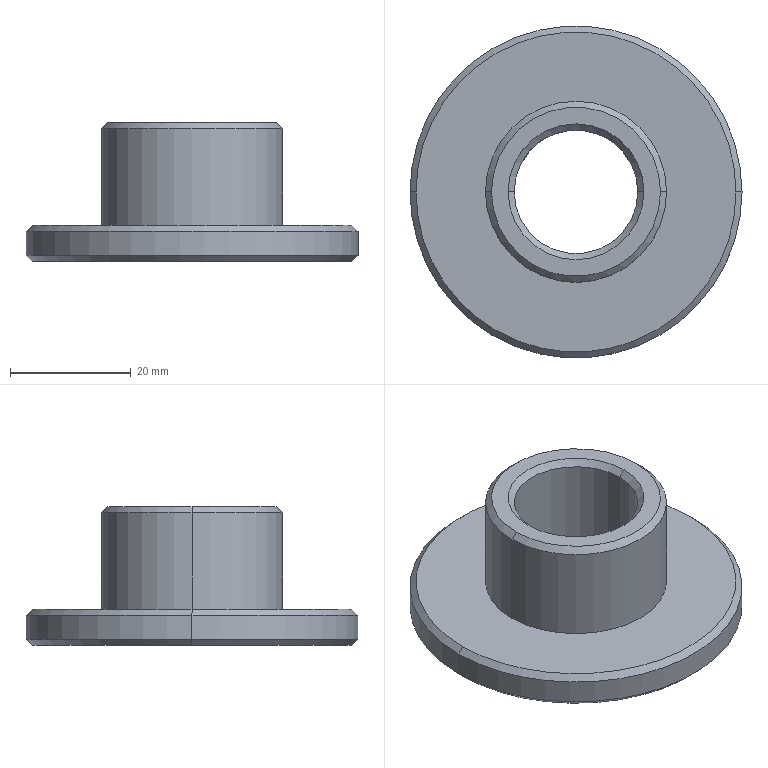Part | STEP file | YCD14007A-08.02.19 Lifting Cylinder Joint Modified | 1 solid | 19 faces | box 55 x 55 x 23 mm | volume 18397 mm3 | cone 10 | cylinder 6 | plane 3 | commonest cylinder face diameters 20.5 x2 30 x2 55 x2
STEP:
#1=CARTESIAN_POINT('',(0.,0.,0.));
#2=DIRECTION('',(0.,0.,1.));
#3=DIRECTION('',(1.,0.,0.));
#4=AXIS2_PLACEMENT_3D('',#1,#2,#3);
#5=CARTESIAN_POINT('',(10.25,0.,10.5));
#6=VERTEX_POINT('',#5);
#7=CARTESIAN_POINT('',(11.25,0.,11.5));
#8=VERTEX_POINT('',#7);
#9=CARTESIAN_POINT('',(10.25,0.,10.5));
#10=DIRECTION('',(0.7071,0.,0.7071));
#11=VECTOR('',#10,1.);
#12=LINE('',#9,#11);
#13=CARTESIAN_POINT('',(0.,0.,10.5));
#14=DIRECTION('',(0.,0.,1.));
#15=DIRECTION('',(1.,0.,0.));
#16=AXIS2_PLACEMENT_3D('',#13,#14,#15);
#17=CONICAL_SURFACE('',#16,10.25,0.7854);
#18=CARTESIAN_POINT('',(6.283,0.));
#19=DIRECTION('',(0.,1.));
#20=VECTOR('',#19,1.);
#21=LINE('',#18,#20);
#22=(GEOMETRIC_REPRESENTATION_CONTEXT(2)PARAMETRIC_REPRESENTATION_CONTEXT()REPRESENTATION_CONTEXT('',''));
#23=DEFINITIONAL_REPRESENTATION('',(#21),#22);
#24=PCURVE('',#17,#23);
#25=CARTESIAN_POINT('',(0.,0.,10.5));
#26=DIRECTION('',(0.,0.,1.));
#27=DIRECTION('',(1.,0.,0.));
#28=AXIS2_PLACEMENT_3D('',#25,#26,#27);
#29=CONICAL_SURFACE('',#28,10.25,0.7854);
#30=CARTESIAN_POINT('',(0.,0.));
#31=DIRECTION('',(0.,1.));
#32=VECTOR('',#31,1.);
#33=LINE('',#30,#32);
#34=(GEOMETRIC_REPRESENTATION_CONTEXT(2)PARAMETRIC_REPRESENTATION_CONTEXT()REPRESENTATION_CONTEXT('',''));
#35=DEFINITIONAL_REPRESENTATION('',(#33),#34);
#36=PCURVE('',#29,#35);
#37=SURFACE_CURVE('',#12,(#24,#36),.PCURVE_S1.);
#38=EDGE_CURVE('',#6,#8,#37,.T.);
#39=ORIENTED_EDGE('',*,*,#38,.T.);
#40=CARTESIAN_POINT('',(-11.25,0.,11.5));
#41=VERTEX_POINT('',#40);
#42=CARTESIAN_POINT('',(0.,0.,11.5));
#43=DIRECTION('',(0.,0.,-1.));
#44=DIRECTION('',(1.,0.,0.));
#45=AXIS2_PLACEMENT_3D('',#42,#43,#44);
#46=CIRCLE('',#45,11.25);
#47=CARTESIAN_POINT('',(6.283,1.));
#48=DIRECTION('',(-1.,0.));
#49=VECTOR('',#48,1.);
#50=LINE('',#47,#49);
#51=(GEOMETRIC_REPRESENTATION_CONTEXT(2)PARAMETRIC_REPRESENTATION_CONTEXT()REPRESENTATION_CONTEXT('',''));
#52=DEFINITIONAL_REPRESENTATION('',(#50),#51);
#53=PCURVE('',#17,#52);
#54=CARTESIAN_POINT('',(10.25,0.,11.5));
#55=DIRECTION('',(0.,0.,1.));
#56=DIRECTION('',(1.,0.,0.));
#57=AXIS2_PLACEMENT_3D('',#54,#55,#56);
#58=PLANE('',#57);
#59=CARTESIAN_POINT('',(1.,0.));
#60=CARTESIAN_POINT('',(1.,-19.486));
#61=CARTESIAN_POINT('',(-15.875,-9.743));
#62=CARTESIAN_POINT('',(-32.75,0.));
#63=CARTESIAN_POINT('',(-15.875,9.743));
#64=CARTESIAN_POINT('',(1.,19.486));
#65=CARTESIAN_POINT('',(1.,0.));
#66=(BOUNDED_CURVE()B_SPLINE_CURVE(2,(#59,#60,#61,#62,#63,#64,#65),.UNSPECIFIED.,.T.,.F.)B_SPLINE_CURVE_WITH_KNOTS((1,2,2,2,2,1),(-2.094,0.,2.094,4.189,6.283,8.378),.UNSPECIFIED.)CURVE()GEOMETRIC_REPRESENTATION_ITEM()RATIONAL_B_SPLINE_CURVE((1.,0.5,1.,0.5,1.,0.5,1.))REPRESENTATION_ITEM(''));
#67=(GEOMETRIC_REPRESENTATION_CONTEXT(2)PARAMETRIC_REPRESENTATION_CONTEXT()REPRESENTATION_CONTEXT('',''));
#68=DEFINITIONAL_REPRESENTATION('',(#66),#67);
#69=PCURVE('',#58,#68);
#70=SURFACE_CURVE('',#46,(#53,#69),.PCURVE_S1.);
#71=EDGE_CURVE('',#8,#41,#70,.T.);
#72=ORIENTED_EDGE('',*,*,#71,.T.);
#73=CARTESIAN_POINT('',(-10.25,0.,10.5));
#74=VERTEX_POINT('',#73);
#75=CARTESIAN_POINT('',(-10.25,0.,10.5));
#76=DIRECTION('',(-0.7071,0.,0.7071));
#77=VECTOR('',#76,1.);
#78=LINE('',#75,#77);
#79=CARTESIAN_POINT('',(3.142,0.));
#80=DIRECTION('',(0.,1.));
#81=VECTOR('',#80,1.);
#82=LINE('',#79,#81);
#83=(GEOMETRIC_REPRESENTATION_CONTEXT(2)PARAMETRIC_REPRESENTATION_CONTEXT()REPRESENTATION_CONTEXT('',''));
#84=DEFINITIONAL_REPRESENTATION('',(#82),#83);
#85=PCURVE('',#17,#84);
#86=CARTESIAN_POINT('',(3.142,0.));
#87=DIRECTION('',(0.,1.));
#88=VECTOR('',#87,1.);
#89=LINE('',#86,#88);
#90=(GEOMETRIC_REPRESENTATION_CONTEXT(2)PARAMETRIC_REPRESENTATION_CONTEXT()REPRESENTATION_CONTEXT('',''));
#91=DEFINITIONAL_REPRESENTATION('',(#89),#90);
#92=PCURVE('',#29,#91);
#93=SURFACE_CURVE('',#78,(#85,#92),.PCURVE_S1.);
#94=EDGE_CURVE('',#74,#41,#93,.T.);
#95=ORIENTED_EDGE('',*,*,#94,.F.);
#96=CARTESIAN_POINT('',(0.,0.,10.5));
#97=DIRECTION('',(0.,0.,1.));
#98=DIRECTION('',(1.,0.,0.));
#99=AXIS2_PLACEMENT_3D('',#96,#97,#98);
#100=CIRCLE('',#99,10.25);
#101=CARTESIAN_POINT('',(0.,0.));
#102=DIRECTION('',(1.,0.));
#103=VECTOR('',#102,1.);
#104=LINE('',#101,#103);
#105=(GEOMETRIC_REPRESENTATION_CONTEXT(2)PARAMETRIC_REPRESENTATION_CONTEXT()REPRESENTATION_CONTEXT('',''));
#106=DEFINITIONAL_REPRESENTATION('',(#104),#105);
#107=PCURVE('',#17,#106);
#108=CARTESIAN_POINT('',(0.,0.,1000.));
#109=DIRECTION('',(0.,0.,1.));
#110=DIRECTION('',(1.,0.,0.));
#111=AXIS2_PLACEMENT_3D('',#108,#109,#110);
#112=CYLINDRICAL_SURFACE('',#111,10.25);
#113=CARTESIAN_POINT('',(0.,-989.5));
#114=DIRECTION('',(1.,0.));
#115=VECTOR('',#114,1.);
#116=LINE('',#113,#115);
#117=(GEOMETRIC_REPRESENTATION_CONTEXT(2)PARAMETRIC_REPRESENTATION_CONTEXT()REPRESENTATION_CONTEXT('',''));
#118=DEFINITIONAL_REPRESENTATION('',(#116),#117);
#119=PCURVE('',#112,#118);
#120=SURFACE_CURVE('',#100,(#107,#119),.PCURVE_S1.);
#121=EDGE_CURVE('',#74,#6,#120,.T.);
#122=ORIENTED_EDGE('',*,*,#121,.T.);
#123=EDGE_LOOP('',(#39,#72,#95,#122));
#124=FACE_BOUND('',#123,.F.);
#125=ADVANCED_FACE('',(#124),#17,.F.);
#126=CARTESIAN_POINT('',(-10.25,0.,-10.5));
#127=VERTEX_POINT('',#126);
#128=CARTESIAN_POINT('',(-11.25,0.,-11.5));
#129=VERTEX_POINT('',#128);
#130=CARTESIAN_POINT('',(-11.25,0.,-11.5));
#131=DIRECTION('',(-0.7071,0.,-0.7071));
#132=VECTOR('',#131,1.);
#133=LINE('',#130,#132);
#134=CARTESIAN_POINT('',(0.,0.,-11.5));
#135=DIRECTION('',(0.,0.,-1.));
#136=DIRECTION('',(-1.,0.,0.));
#137=AXIS2_PLACEMENT_3D('',#134,#135,#136);
#138=CONICAL_SURFACE('',#137,11.25,0.7854);
#139=CARTESIAN_POINT('',(6.283,0.));
#140=DIRECTION('',(0.,1.));
#141=VECTOR('',#140,1.);
#142=LINE('',#139,#141);
#143=(GEOMETRIC_REPRESENTATION_CONTEXT(2)PARAMETRIC_REPRESENTATION_CONTEXT()REPRESENTATION_CONTEXT('',''));
#144=DEFINITIONAL_REPRESENTATION('',(#142),#143);
#145=PCURVE('',#138,#144);
#146=CARTESIAN_POINT('',(0.,0.,-11.5));
#147=DIRECTION('',(0.,0.,-1.));
#148=DIRECTION('',(-1.,0.,0.));
#149=AXIS2_PLACEMENT_3D('',#146,#147,#148);
#150=CONICAL_SURFACE('',#149,11.25,0.7854);
#151=CARTESIAN_POINT('',(0.,0.));
#152=DIRECTION('',(0.,1.));
#153=VECTOR('',#152,1.);
#154=LINE('',#151,#153);
#155=(GEOMETRIC_REPRESENTATION_CONTEXT(2)PARAMETRIC_REPRESENTATION_CONTEXT()REPRESENTATION_CONTEXT('',''));
#156=DEFINITIONAL_REPRESENTATION('',(#154),#155);
#157=PCURVE('',#150,#156);
#158=SURFACE_CURVE('',#133,(#145,#157),.PCURVE_S1.);
#159=EDGE_CURVE('',#127,#129,#158,.T.);
#160=ORIENTED_EDGE('',*,*,#159,.T.);
#161=CARTESIAN_POINT('',(11.25,0.,-11.5));
#162=VERTEX_POINT('',#161);
#163=CARTESIAN_POINT('',(0.,0.,-11.5));
#164=DIRECTION('',(0.,0.,1.));
#165=DIRECTION('',(-1.,0.,0.));
#166=AXIS2_PLACEMENT_3D('',#163,#164,#165);
#167=CIRCLE('',#166,11.25);
#168=CARTESIAN_POINT('',(6.283,0.));
#169=DIRECTION('',(-1.,0.));
#170=VECTOR('',#169,1.);
#171=LINE('',#168,#170);
#172=(GEOMETRIC_REPRESENTATION_CONTEXT(2)PARAMETRIC_REPRESENTATION_CONTEXT()REPRESENTATION_CONTEXT('',''));
#173=DEFINITIONAL_REPRESENTATION('',(#171),#172);
#174=PCURVE('',#138,#173);
#175=CARTESIAN_POINT('',(27.5,0.,-11.5));
#176=DIRECTION('',(0.,0.,-1.));
#177=DIRECTION('',(-1.,0.,0.));
#178=AXIS2_PLACEMENT_3D('',#175,#176,#177);
#179=PLANE('',#178);
#180=CARTESIAN_POINT('',(38.75,0.));
#181=CARTESIAN_POINT('',(38.75,-19.486));
#182=CARTESIAN_POINT('',(21.875,-9.743));
#183=CARTESIAN_POINT('',(5.,0.));
#184=CARTESIAN_POINT('',(21.875,9.743));
#185=CARTESIAN_POINT('',(38.75,19.486));
#186=CARTESIAN_POINT('',(38.75,0.));
#187=(BOUNDED_CURVE()B_SPLINE_CURVE(2,(#180,#181,#182,#183,#184,#185,#186),.UNSPECIFIED.,.T.,.F.)B_SPLINE_CURVE_WITH_KNOTS((1,2,2,2,2,1),(-2.094,0.,2.094,4.189,6.283,8.378),.UNSPECIFIED.)CURVE()GEOMETRIC_REPRESENTATION_ITEM()RATIONAL_B_SPLINE_CURVE((1.,0.5,1.,0.5,1.,0.5,1.))REPRESENTATION_ITEM(''));
#188=(GEOMETRIC_REPRESENTATION_CONTEXT(2)PARAMETRIC_REPRESENTATION_CONTEXT()REPRESENTATION_CONTEXT('',''));
#189=DEFINITIONAL_REPRESENTATION('',(#187),#188);
#190=PCURVE('',#179,#189);
#191=SURFACE_CURVE('',#167,(#174,#190),.PCURVE_S1.);
#192=EDGE_CURVE('',#129,#162,#191,.T.);
#193=ORIENTED_EDGE('',*,*,#192,.T.);
#194=CARTESIAN_POINT('',(10.25,0.,-10.5));
#195=VERTEX_POINT('',#194);
#196=CARTESIAN_POINT('',(11.25,0.,-11.5));
#197=DIRECTION('',(0.7071,0.,-0.7071));
#198=VECTOR('',#197,1.);
#199=LINE('',#196,#198);
#200=CARTESIAN_POINT('',(3.142,0.));
#201=DIRECTION('',(0.,1.));
#202=VECTOR('',#201,1.);
#203=LINE('',#200,#202);
#204=(GEOMETRIC_REPRESENTATION_CONTEXT(2)PARAMETRIC_REPRESENTATION_CONTEXT()REPRESENTATION_CONTEXT('',''));
#205=DEFINITIONAL_REPRESENTATION('',(#203),#204);
#206=PCURVE('',#138,#205);
#207=CARTESIAN_POINT('',(3.142,0.));
#208=DIRECTION('',(0.,1.));
#209=VECTOR('',#208,1.);
#210=LINE('',#207,#209);
#211=(GEOMETRIC_REPRESENTATION_CONTEXT(2)PARAMETRIC_REPRESENTATION_CONTEXT()REPRESENTATION_CONTEXT('',''));
#212=DEFINITIONAL_REPRESENTATION('',(#210),#211);
#213=PCURVE('',#150,#212);
#214=SURFACE_CURVE('',#199,(#206,#213),.PCURVE_S1.);
#215=EDGE_CURVE('',#195,#162,#214,.T.);
#216=ORIENTED_EDGE('',*,*,#215,.F.);
#217=CARTESIAN_POINT('',(0.,0.,-10.5));
#218=DIRECTION('',(0.,0.,-1.));
#219=DIRECTION('',(-1.,0.,0.));
#220=AXIS2_PLACEMENT_3D('',#217,#218,#219);
#221=CIRCLE('',#220,10.25);
#222=CARTESIAN_POINT('',(0.,-1.));
#223=DIRECTION('',(1.,0.));
#224=VECTOR('',#223,1.);
#225=LINE('',#222,#224);
#226=(GEOMETRIC_REPRESENTATION_CONTEXT(2)PARAMETRIC_REPRESENTATION_CONTEXT()REPRESENTATION_CONTEXT('',''));
#227=DEFINITIONAL_REPRESENTATION('',(#225),#226);
#228=PCURVE('',#138,#227);
#229=CARTESIAN_POINT('',(9.425,-1010.5));
#230=DIRECTION('',(-1.,0.));
#231=VECTOR('',#230,1.);
#232=LINE('',#229,#231);
#233=(GEOMETRIC_REPRESENTATION_CONTEXT(2)PARAMETRIC_REPRESENTATION_CONTEXT()REPRESENTATION_CONTEXT('',''));
#234=DEFINITIONAL_REPRESENTATION('',(#232),#233);
#235=PCURVE('',#112,#234);
#236=SURFACE_CURVE('',#221,(#228,#235),.PCURVE_S1.);
#237=EDGE_CURVE('',#195,#127,#236,.T.);
#238=ORIENTED_EDGE('',*,*,#237,.T.);
#239=EDGE_LOOP('',(#160,#193,#216,#238));
#240=FACE_BOUND('',#239,.F.);
#241=ADVANCED_FACE('',(#240),#138,.F.);
#242=CARTESIAN_POINT('',(-26.5,0.,-11.5));
#243=VERTEX_POINT('',#242);
#244=CARTESIAN_POINT('',(26.5,0.,-11.5));
#245=VERTEX_POINT('',#244);
#246=CARTESIAN_POINT('',(0.,0.,-11.5));
#247=DIRECTION('',(0.,0.,-1.));
#248=DIRECTION('',(-1.,0.,0.));
#249=AXIS2_PLACEMENT_3D('',#246,#247,#248);
#250=CIRCLE('',#249,26.5);
#251=CARTESIAN_POINT('',(0.,0.,-10.5));
#252=DIRECTION('',(0.,0.,1.));
#253=DIRECTION('',(1.,0.,0.));
#254=AXIS2_PLACEMENT_3D('',#251,#252,#253);
#255=CONICAL_SURFACE('',#254,27.5,0.7854);
#256=CARTESIAN_POINT('',(3.142,-1.));
#257=DIRECTION('',(-1.,0.));
#258=VECTOR('',#257,1.);
#259=LINE('',#256,#258);
#260=(GEOMETRIC_REPRESENTATION_CONTEXT(2)PARAMETRIC_REPRESENTATION_CONTEXT()REPRESENTATION_CONTEXT('',''));
#261=DEFINITIONAL_REPRESENTATION('',(#259),#260);
#262=PCURVE('',#255,#261);
#263=CARTESIAN_POINT('',(27.5,0.));
#264=DIRECTION('',(1.,0.));
#265=AXIS2_PLACEMENT_2D('',#263,#264);
#266=CIRCLE('',#265,26.5);
#267=(GEOMETRIC_REPRESENTATION_CONTEXT(2)PARAMETRIC_REPRESENTATION_CONTEXT()REPRESENTATION_CONTEXT('',''));
#268=DEFINITIONAL_REPRESENTATION('',(#266),#267);
#269=PCURVE('',#179,#268);
#270=SURFACE_CURVE('',#250,(#262,#269),.PCURVE_S1.);
#271=EDGE_CURVE('',#243,#245,#270,.T.);
#272=ORIENTED_EDGE('',*,*,#271,.F.);
#273=CARTESIAN_POINT('',(-27.5,0.,-10.5));
#274=VERTEX_POINT('',#273);
#275=CARTESIAN_POINT('',(-27.5,0.,-10.5));
#276=DIRECTION('',(-0.7071,0.,0.7071));
#277=VECTOR('',#276,1.);
#278=LINE('',#275,#277);
#279=CARTESIAN_POINT('',(3.142,0.));
#280=DIRECTION('',(0.,1.));
#281=VECTOR('',#280,1.);
#282=LINE('',#279,#281);
#283=(GEOMETRIC_REPRESENTATION_CONTEXT(2)PARAMETRIC_REPRESENTATION_CONTEXT()REPRESENTATION_CONTEXT('',''));
#284=DEFINITIONAL_REPRESENTATION('',(#282),#283);
#285=PCURVE('',#255,#284);
#286=CARTESIAN_POINT('',(0.,0.,-10.5));
#287=DIRECTION('',(0.,0.,1.));
#288=DIRECTION('',(1.,0.,0.));
#289=AXIS2_PLACEMENT_3D('',#286,#287,#288);
#290=CONICAL_SURFACE('',#289,27.5,0.7854);
#291=CARTESIAN_POINT('',(3.142,0.));
#292=DIRECTION('',(0.,1.));
#293=VECTOR('',#292,1.);
#294=LINE('',#291,#293);
#295=(GEOMETRIC_REPRESENTATION_CONTEXT(2)PARAMETRIC_REPRESENTATION_CONTEXT()REPRESENTATION_CONTEXT('',''));
#296=DEFINITIONAL_REPRESENTATION('',(#294),#295);
#297=PCURVE('',#290,#296);
#298=SURFACE_CURVE('',#278,(#285,#297),.PCURVE_S1.);
#299=EDGE_CURVE('',#243,#274,#298,.T.);
#300=ORIENTED_EDGE('',*,*,#299,.T.);
#301=CARTESIAN_POINT('',(27.5,0.,-10.5));
#302=VERTEX_POINT('',#301);
#303=CARTESIAN_POINT('',(0.,0.,-10.5));
#304=DIRECTION('',(0.,0.,1.));
#305=DIRECTION('',(-1.,0.,0.));
#306=AXIS2_PLACEMENT_3D('',#303,#304,#305);
#307=CIRCLE('',#306,27.5);
#308=CARTESIAN_POINT('',(-3.142,0.));
#309=DIRECTION('',(1.,0.));
#310=VECTOR('',#309,1.);
#311=LINE('',#308,#310);
#312=(GEOMETRIC_REPRESENTATION_CONTEXT(2)PARAMETRIC_REPRESENTATION_CONTEXT()REPRESENTATION_CONTEXT('',''));
#313=DEFINITIONAL_REPRESENTATION('',(#311),#312);
#314=PCURVE('',#255,#313);
#315=CARTESIAN_POINT('',(0.,0.,1000.));
#316=DIRECTION('',(0.,0.,1.));
#317=DIRECTION('',(1.,0.,0.));
#318=AXIS2_PLACEMENT_3D('',#315,#316,#317);
#319=CYLINDRICAL_SURFACE('',#318,27.5);
#320=CARTESIAN_POINT('',(-3.142,-1010.5));
#321=DIRECTION('',(1.,0.));
#322=VECTOR('',#321,1.);
#323=LINE('',#320,#322);
#324=(GEOMETRIC_REPRESENTATION_CONTEXT(2)PARAMETRIC_REPRESENTATION_CONTEXT()REPRESENTATION_CONTEXT('',''));
#325=DEFINITIONAL_REPRESENTATION('',(#323),#324);
#326=PCURVE('',#319,#325);
#327=SURFACE_CURVE('',#307,(#314,#326),.PCURVE_S1.);
#328=EDGE_CURVE('',#302,#274,#327,.T.);
#329=ORIENTED_EDGE('',*,*,#328,.F.);
#330=CARTESIAN_POINT('',(27.5,0.,-10.5));
#331=DIRECTION('',(0.7071,0.,0.7071));
#332=VECTOR('',#331,1.);
#333=LINE('',#330,#332);
#334=CARTESIAN_POINT('',(0.,0.));
#335=DIRECTION('',(0.,1.));
#336=VECTOR('',#335,1.);
#337=LINE('',#334,#336);
#338=(GEOMETRIC_REPRESENTATION_CONTEXT(2)PARAMETRIC_REPRESENTATION_CONTEXT()REPRESENTATION_CONTEXT('',''));
#339=DEFINITIONAL_REPRESENTATION('',(#337),#338);
#340=PCURVE('',#255,#339);
#341=CARTESIAN_POINT('',(6.283,0.));
#342=DIRECTION('',(0.,1.));
#343=VECTOR('',#342,1.);
#344=LINE('',#341,#343);
#345=(GEOMETRIC_REPRESENTATION_CONTEXT(2)PARAMETRIC_REPRESENTATION_CONTEXT()REPRESENTATION_CONTEXT('',''));
#346=DEFINITIONAL_REPRESENTATION('',(#344),#345);
#347=PCURVE('',#290,#346);
#348=SURFACE_CURVE('',#333,(#340,#347),.PCURVE_S1.);
#349=EDGE_CURVE('',#245,#302,#348,.T.);
#350=ORIENTED_EDGE('',*,*,#349,.F.);
#351=EDGE_LOOP('',(#272,#300,#329,#350));
#352=FACE_BOUND('',#351,.T.);
#353=ADVANCED_FACE('',(#352),#255,.T.);
#354=CARTESIAN_POINT('',(26.5,0.,-5.5));
#355=VERTEX_POINT('',#354);
#356=CARTESIAN_POINT('',(-26.5,0.,-5.5));
#357=VERTEX_POINT('',#356);
#358=CARTESIAN_POINT('',(0.,0.,-5.5));
#359=DIRECTION('',(0.,0.,1.));
#360=DIRECTION('',(1.,0.,0.));
#361=AXIS2_PLACEMENT_3D('',#358,#359,#360);
#362=CIRCLE('',#361,26.5);
#363=CARTESIAN_POINT('',(0.,0.,-5.5));
#364=DIRECTION('',(0.,0.,-1.));
#365=DIRECTION('',(-1.,0.,0.));
#366=AXIS2_PLACEMENT_3D('',#363,#364,#365);
#367=CONICAL_SURFACE('',#366,26.5,0.7854);
#368=CARTESIAN_POINT('',(3.142,0.));
#369=DIRECTION('',(-1.,0.));
#370=VECTOR('',#369,1.);
#371=LINE('',#368,#370);
#372=(GEOMETRIC_REPRESENTATION_CONTEXT(2)PARAMETRIC_REPRESENTATION_CONTEXT()REPRESENTATION_CONTEXT('',''));
#373=DEFINITIONAL_REPRESENTATION('',(#371),#372);
#374=PCURVE('',#367,#373);
#375=CARTESIAN_POINT('',(15.,0.,-5.5));
#376=DIRECTION('',(0.,0.,1.));
#377=DIRECTION('',(1.,0.,0.));
#378=AXIS2_PLACEMENT_3D('',#375,#376,#377);
#379=PLANE('',#378);
#380=CARTESIAN_POINT('',(-15.,0.));
#381=DIRECTION('',(1.,0.));
#382=AXIS2_PLACEMENT_2D('',#380,#381);
#383=CIRCLE('',#382,26.5);
#384=(GEOMETRIC_REPRESENTATION_CONTEXT(2)PARAMETRIC_REPRESENTATION_CONTEXT()REPRESENTATION_CONTEXT('',''));
#385=DEFINITIONAL_REPRESENTATION('',(#383),#384);
#386=PCURVE('',#379,#385);
#387=SURFACE_CURVE('',#362,(#374,#386),.PCURVE_S1.);
#388=EDGE_CURVE('',#355,#357,#387,.T.);
#389=ORIENTED_EDGE('',*,*,#388,.F.);
#390=CARTESIAN_POINT('',(27.5,0.,-6.5));
#391=VERTEX_POINT('',#390);
#392=CARTESIAN_POINT('',(26.5,0.,-5.5));
#393=DIRECTION('',(0.7071,0.,-0.7071));
#394=VECTOR('',#393,1.);
#395=LINE('',#392,#394);
#396=CARTESIAN_POINT('',(3.142,0.));
#397=DIRECTION('',(0.,1.));
#398=VECTOR('',#397,1.);
#399=LINE('',#396,#398);
#400=(GEOMETRIC_REPRESENTATION_CONTEXT(2)PARAMETRIC_REPRESENTATION_CONTEXT()REPRESENTATION_CONTEXT('',''));
#401=DEFINITIONAL_REPRESENTATION('',(#399),#400);
#402=PCURVE('',#367,#401);
#403=CARTESIAN_POINT('',(0.,0.,-5.5));
#404=DIRECTION('',(0.,0.,-1.));
#405=DIRECTION('',(-1.,0.,0.));
#406=AXIS2_PLACEMENT_3D('',#403,#404,#405);
#407=CONICAL_SURFACE('',#406,26.5,0.7854);
#408=CARTESIAN_POINT('',(3.142,0.));
#409=DIRECTION('',(0.,1.));
#410=VECTOR('',#409,1.);
#411=LINE('',#408,#410);
#412=(GEOMETRIC_REPRESENTATION_CONTEXT(2)PARAMETRIC_REPRESENTATION_CONTEXT()REPRESENTATION_CONTEXT('',''));
#413=DEFINITIONAL_REPRESENTATION('',(#411),#412);
#414=PCURVE('',#407,#413);
#415=SURFACE_CURVE('',#395,(#402,#414),.PCURVE_S1.);
#416=EDGE_CURVE('',#355,#391,#415,.T.);
#417=ORIENTED_EDGE('',*,*,#416,.T.);
#418=CARTESIAN_POINT('',(-27.5,0.,-6.5));
#419=VERTEX_POINT('',#418);
#420=CARTESIAN_POINT('',(0.,0.,-6.5));
#421=DIRECTION('',(0.,0.,-1.));
#422=DIRECTION('',(1.,0.,0.));
#423=AXIS2_PLACEMENT_3D('',#420,#421,#422);
#424=CIRCLE('',#423,27.5);
#425=CARTESIAN_POINT('',(-3.142,1.));
#426=DIRECTION('',(1.,0.));
#427=VECTOR('',#426,1.);
#428=LINE('',#425,#427);
#429=(GEOMETRIC_REPRESENTATION_CONTEXT(2)PARAMETRIC_REPRESENTATION_CONTEXT()REPRESENTATION_CONTEXT('',''));
#430=DEFINITIONAL_REPRESENTATION('',(#428),#429);
#431=PCURVE('',#367,#430);
#432=CARTESIAN_POINT('',(6.283,-1006.5));
#433=DIRECTION('',(-1.,0.));
#434=VECTOR('',#433,1.);
#435=LINE('',#432,#434);
#436=(GEOMETRIC_REPRESENTATION_CONTEXT(2)PARAMETRIC_REPRESENTATION_CONTEXT()REPRESENTATION_CONTEXT('',''));
#437=DEFINITIONAL_REPRESENTATION('',(#435),#436);
#438=PCURVE('',#319,#437);
#439=SURFACE_CURVE('',#424,(#431,#438),.PCURVE_S1.);
#440=EDGE_CURVE('',#419,#391,#439,.T.);
#441=ORIENTED_EDGE('',*,*,#440,.F.);
#442=CARTESIAN_POINT('',(-26.5,0.,-5.5));
#443=DIRECTION('',(-0.7071,0.,-0.7071));
#444=VECTOR('',#443,1.);
#445=LINE('',#442,#444);
#446=CARTESIAN_POINT('',(0.,0.));
#447=DIRECTION('',(0.,1.));
#448=VECTOR('',#447,1.);
#449=LINE('',#446,#448);
#450=(GEOMETRIC_REPRESENTATION_CONTEXT(2)PARAMETRIC_REPRESENTATION_CONTEXT()REPRESENTATION_CONTEXT('',''));
#451=DEFINITIONAL_REPRESENTATION('',(#449),#450);
#452=PCURVE('',#367,#451);
#453=CARTESIAN_POINT('',(6.283,0.));
#454=DIRECTION('',(0.,1.));
#455=VECTOR('',#454,1.);
#456=LINE('',#453,#455);
#457=(GEOMETRIC_REPRESENTATION_CONTEXT(2)PARAMETRIC_REPRESENTATION_CONTEXT()REPRESENTATION_CONTEXT('',''));
#458=DEFINITIONAL_REPRESENTATION('',(#456),#457);
#459=PCURVE('',#407,#458);
#460=SURFACE_CURVE('',#445,(#452,#459),.PCURVE_S1.);
#461=EDGE_CURVE('',#357,#419,#460,.T.);
#462=ORIENTED_EDGE('',*,*,#461,.F.);
#463=EDGE_LOOP('',(#389,#417,#441,#462));
#464=FACE_BOUND('',#463,.T.);
#465=ADVANCED_FACE('',(#464),#367,.T.);
#466=CARTESIAN_POINT('',(14.,0.,11.5));
#467=VERTEX_POINT('',#466);
#468=CARTESIAN_POINT('',(-14.,0.,11.5));
#469=VERTEX_POINT('',#468);
#470=CARTESIAN_POINT('',(0.,0.,11.5));
#471=DIRECTION('',(0.,0.,1.));
#472=DIRECTION('',(1.,0.,0.));
#473=AXIS2_PLACEMENT_3D('',#470,#471,#472);
#474=CIRCLE('',#473,14.);
#475=CARTESIAN_POINT('',(0.,0.,11.5));
#476=DIRECTION('',(0.,0.,-1.));
#477=DIRECTION('',(-1.,0.,0.));
#478=AXIS2_PLACEMENT_3D('',#475,#476,#477);
#479=CONICAL_SURFACE('',#478,14.,0.7854);
#480=CARTESIAN_POINT('',(3.142,0.));
#481=DIRECTION('',(-1.,0.));
#482=VECTOR('',#481,1.);
#483=LINE('',#480,#482);
#484=(GEOMETRIC_REPRESENTATION_CONTEXT(2)PARAMETRIC_REPRESENTATION_CONTEXT()REPRESENTATION_CONTEXT('',''));
#485=DEFINITIONAL_REPRESENTATION('',(#483),#484);
#486=PCURVE('',#479,#485);
#487=CARTESIAN_POINT('',(-10.25,0.));
#488=DIRECTION('',(1.,0.));
#489=AXIS2_PLACEMENT_2D('',#487,#488);
#490=CIRCLE('',#489,14.);
#491=(GEOMETRIC_REPRESENTATION_CONTEXT(2)PARAMETRIC_REPRESENTATION_CONTEXT()REPRESENTATION_CONTEXT('',''));
#492=DEFINITIONAL_REPRESENTATION('',(#490),#491);
#493=PCURVE('',#58,#492);
#494=SURFACE_CURVE('',#474,(#486,#493),.PCURVE_S1.);
#495=EDGE_CURVE('',#467,#469,#494,.T.);
#496=ORIENTED_EDGE('',*,*,#495,.F.);
#497=CARTESIAN_POINT('',(15.,0.,10.5));
#498=VERTEX_POINT('',#497);
#499=CARTESIAN_POINT('',(14.,0.,11.5));
#500=DIRECTION('',(0.7071,0.,-0.7071));
#501=VECTOR('',#500,1.);
#502=LINE('',#499,#501);
#503=CARTESIAN_POINT('',(3.142,0.));
#504=DIRECTION('',(0.,1.));
#505=VECTOR('',#504,1.);
#506=LINE('',#503,#505);
#507=(GEOMETRIC_REPRESENTATION_CONTEXT(2)PARAMETRIC_REPRESENTATION_CONTEXT()REPRESENTATION_CONTEXT('',''));
#508=DEFINITIONAL_REPRESENTATION('',(#506),#507);
#509=PCURVE('',#479,#508);
#510=CARTESIAN_POINT('',(0.,0.,11.5));
#511=DIRECTION('',(0.,0.,-1.));
#512=DIRECTION('',(-1.,0.,0.));
#513=AXIS2_PLACEMENT_3D('',#510,#511,#512);
#514=CONICAL_SURFACE('',#513,14.,0.7854);
#515=CARTESIAN_POINT('',(3.142,0.));
#516=DIRECTION('',(0.,1.));
#517=VECTOR('',#516,1.);
#518=LINE('',#515,#517);
#519=(GEOMETRIC_REPRESENTATION_CONTEXT(2)PARAMETRIC_REPRESENTATION_CONTEXT()REPRESENTATION_CONTEXT('',''));
#520=DEFINITIONAL_REPRESENTATION('',(#518),#519);
#521=PCURVE('',#514,#520);
#522=SURFACE_CURVE('',#502,(#509,#521),.PCURVE_S1.);
#523=EDGE_CURVE('',#467,#498,#522,.T.);
#524=ORIENTED_EDGE('',*,*,#523,.T.);
#525=CARTESIAN_POINT('',(-15.,0.,10.5));
#526=VERTEX_POINT('',#525);
#527=CARTESIAN_POINT('',(0.,0.,10.5));
#528=DIRECTION('',(0.,0.,-1.));
#529=DIRECTION('',(1.,0.,0.));
#530=AXIS2_PLACEMENT_3D('',#527,#528,#529);
#531=CIRCLE('',#530,15.);
#532=CARTESIAN_POINT('',(-3.142,1.));
#533=DIRECTION('',(1.,0.));
#534=VECTOR('',#533,1.);
#535=LINE('',#532,#534);
#536=(GEOMETRIC_REPRESENTATION_CONTEXT(2)PARAMETRIC_REPRESENTATION_CONTEXT()REPRESENTATION_CONTEXT('',''));
#537=DEFINITIONAL_REPRESENTATION('',(#535),#536);
#538=PCURVE('',#479,#537);
#539=CARTESIAN_POINT('',(0.,0.,1000.));
#540=DIRECTION('',(0.,0.,1.));
#541=DIRECTION('',(1.,0.,0.));
#542=AXIS2_PLACEMENT_3D('',#539,#540,#541);
#543=CYLINDRICAL_SURFACE('',#542,15.);
#544=CARTESIAN_POINT('',(6.283,-989.5));
#545=DIRECTION('',(-1.,0.));
#546=VECTOR('',#545,1.);
#547=LINE('',#544,#546);
#548=(GEOMETRIC_REPRESENTATION_CONTEXT(2)PARAMETRIC_REPRESENTATION_CONTEXT()REPRESENTATION_CONTEXT('',''));
#549=DEFINITIONAL_REPRESENTATION('',(#547),#548);
#550=PCURVE('',#543,#549);
#551=SURFACE_CURVE('',#531,(#538,#550),.PCURVE_S1.);
#552=EDGE_CURVE('',#526,#498,#551,.T.);
#553=ORIENTED_EDGE('',*,*,#552,.F.);
#554=CARTESIAN_POINT('',(-14.,0.,11.5));
#555=DIRECTION('',(-0.7071,0.,-0.7071));
#556=VECTOR('',#555,1.);
#557=LINE('',#554,#556);
#558=CARTESIAN_POINT('',(0.,0.));
#559=DIRECTION('',(0.,1.));
#560=VECTOR('',#559,1.);
#561=LINE('',#558,#560);
#562=(GEOMETRIC_REPRESENTATION_CONTEXT(2)PARAMETRIC_REPRESENTATION_CONTEXT()REPRESENTATION_CONTEXT('',''));
#563=DEFINITIONAL_REPRESENTATION('',(#561),#562);
#564=PCURVE('',#479,#563);
#565=CARTESIAN_POINT('',(6.283,0.));
#566=DIRECTION('',(0.,1.));
#567=VECTOR('',#566,1.);
#568=LINE('',#565,#567);
#569=(GEOMETRIC_REPRESENTATION_CONTEXT(2)PARAMETRIC_REPRESENTATION_CONTEXT()REPRESENTATION_CONTEXT('',''));
#570=DEFINITIONAL_REPRESENTATION('',(#568),#569);
#571=PCURVE('',#514,#570);
#572=SURFACE_CURVE('',#557,(#564,#571),.PCURVE_S1.);
#573=EDGE_CURVE('',#469,#526,#572,.T.);
#574=ORIENTED_EDGE('',*,*,#573,.F.);
#575=EDGE_LOOP('',(#496,#524,#553,#574));
#576=FACE_BOUND('',#575,.T.);
#577=ADVANCED_FACE('',(#576),#479,.T.);
#578=ORIENTED_EDGE('',*,*,#328,.T.);
#579=CARTESIAN_POINT('',(-27.5,0.,1000.));
#580=DIRECTION('',(0.,0.,1.));
#581=VECTOR('',#580,1.);
#582=LINE('',#579,#581);
#583=CARTESIAN_POINT('',(3.142,0.));
#584=DIRECTION('',(0.,1.));
#585=VECTOR('',#584,1.);
#586=LINE('',#583,#585);
#587=(GEOMETRIC_REPRESENTATION_CONTEXT(2)PARAMETRIC_REPRESENTATION_CONTEXT()REPRESENTATION_CONTEXT('',''));
#588=DEFINITIONAL_REPRESENTATION('',(#586),#587);
#589=PCURVE('',#319,#588);
#590=CARTESIAN_POINT('',(0.,0.,1000.));
#591=DIRECTION('',(0.,0.,1.));
#592=DIRECTION('',(1.,0.,0.));
#593=AXIS2_PLACEMENT_3D('',#590,#591,#592);
#594=CYLINDRICAL_SURFACE('',#593,27.5);
#595=CARTESIAN_POINT('',(3.142,0.));
#596=DIRECTION('',(0.,1.));
#597=VECTOR('',#596,1.);
#598=LINE('',#595,#597);
#599=(GEOMETRIC_REPRESENTATION_CONTEXT(2)PARAMETRIC_REPRESENTATION_CONTEXT()REPRESENTATION_CONTEXT('',''));
#600=DEFINITIONAL_REPRESENTATION('',(#598),#599);
#601=PCURVE('',#594,#600);
#602=SURFACE_CURVE('',#582,(#589,#601),.PCURVE_S1.);
#603=EDGE_CURVE('',#274,#419,#602,.T.);
#604=ORIENTED_EDGE('',*,*,#603,.T.);
#605=ORIENTED_EDGE('',*,*,#440,.T.);
#606=CARTESIAN_POINT('',(27.5,0.,1000.));
#607=DIRECTION('',(0.,0.,1.));
#608=VECTOR('',#607,1.);
#609=LINE('',#606,#608);
#610=CARTESIAN_POINT('',(0.,0.));
#611=DIRECTION('',(0.,1.));
#612=VECTOR('',#611,1.);
#613=LINE('',#610,#612);
#614=(GEOMETRIC_REPRESENTATION_CONTEXT(2)PARAMETRIC_REPRESENTATION_CONTEXT()REPRESENTATION_CONTEXT('',''));
#615=DEFINITIONAL_REPRESENTATION('',(#613),#614);
#616=PCURVE('',#319,#615);
#617=CARTESIAN_POINT('',(6.283,0.));
#618=DIRECTION('',(0.,1.));
#619=VECTOR('',#618,1.);
#620=LINE('',#617,#619);
#621=(GEOMETRIC_REPRESENTATION_CONTEXT(2)PARAMETRIC_REPRESENTATION_CONTEXT()REPRESENTATION_CONTEXT('',''));
#622=DEFINITIONAL_REPRESENTATION('',(#620),#621);
#623=PCURVE('',#594,#622);
#624=SURFACE_CURVE('',#609,(#616,#623),.PCURVE_S1.);
#625=EDGE_CURVE('',#302,#391,#624,.T.);
#626=ORIENTED_EDGE('',*,*,#625,.F.);
#627=EDGE_LOOP('',(#578,#604,#605,#626));
#628=FACE_BOUND('',#627,.T.);
#629=ADVANCED_FACE('',(#628),#319,.T.);
#630=CARTESIAN_POINT('',(10.25,0.,1000.));
#631=DIRECTION('',(0.,0.,1.));
#632=VECTOR('',#631,1.);
#633=LINE('',#630,#632);
#634=CARTESIAN_POINT('',(6.283,0.));
#635=DIRECTION('',(0.,1.));
#636=VECTOR('',#635,1.);
#637=LINE('',#634,#636);
#638=(GEOMETRIC_REPRESENTATION_CONTEXT(2)PARAMETRIC_REPRESENTATION_CONTEXT()REPRESENTATION_CONTEXT('',''));
#639=DEFINITIONAL_REPRESENTATION('',(#637),#638);
#640=PCURVE('',#112,#639);
#641=CARTESIAN_POINT('',(0.,0.,1000.));
#642=DIRECTION('',(0.,0.,1.));
#643=DIRECTION('',(1.,0.,0.));
#644=AXIS2_PLACEMENT_3D('',#641,#642,#643);
#645=CYLINDRICAL_SURFACE('',#644,10.25);
#646=CARTESIAN_POINT('',(0.,0.));
#647=DIRECTION('',(0.,1.));
#648=VECTOR('',#647,1.);
#649=LINE('',#646,#648);
#650=(GEOMETRIC_REPRESENTATION_CONTEXT(2)PARAMETRIC_REPRESENTATION_CONTEXT()REPRESENTATION_CONTEXT('',''));
#651=DEFINITIONAL_REPRESENTATION('',(#649),#650);
#652=PCURVE('',#645,#651);
#653=SURFACE_CURVE('',#633,(#640,#652),.PCURVE_S1.);
#654=EDGE_CURVE('',#195,#6,#653,.T.);
#655=ORIENTED_EDGE('',*,*,#654,.T.);
#656=ORIENTED_EDGE('',*,*,#121,.F.);
#657=CARTESIAN_POINT('',(-10.25,0.,1000.));
#658=DIRECTION('',(0.,0.,1.));
#659=VECTOR('',#658,1.);
#660=LINE('',#657,#659);
#661=CARTESIAN_POINT('',(3.142,0.));
#662=DIRECTION('',(0.,1.));
#663=VECTOR('',#662,1.);
#664=LINE('',#661,#663);
#665=(GEOMETRIC_REPRESENTATION_CONTEXT(2)PARAMETRIC_REPRESENTATION_CONTEXT()REPRESENTATION_CONTEXT('',''));
#666=DEFINITIONAL_REPRESENTATION('',(#664),#665);
#667=PCURVE('',#112,#666);
#668=CARTESIAN_POINT('',(3.142,0.));
#669=DIRECTION('',(0.,1.));
#670=VECTOR('',#669,1.);
#671=LINE('',#668,#670);
#672=(GEOMETRIC_REPRESENTATION_CONTEXT(2)PARAMETRIC_REPRESENTATION_CONTEXT()REPRESENTATION_CONTEXT('',''));
#673=DEFINITIONAL_REPRESENTATION('',(#671),#672);
#674=PCURVE('',#645,#673);
#675=SURFACE_CURVE('',#660,(#667,#674),.PCURVE_S1.);
#676=EDGE_CURVE('',#127,#74,#675,.T.);
#677=ORIENTED_EDGE('',*,*,#676,.F.);
#678=ORIENTED_EDGE('',*,*,#237,.F.);
#679=EDGE_LOOP('',(#655,#656,#677,#678));
#680=FACE_BOUND('',#679,.F.);
#681=ADVANCED_FACE('',(#680),#112,.F.);
#682=CARTESIAN_POINT('',(15.,0.,-5.5));
#683=VERTEX_POINT('',#682);
#684=CARTESIAN_POINT('',(-15.,0.,-5.5));
#685=VERTEX_POINT('',#684);
#686=CARTESIAN_POINT('',(0.,0.,-5.5));
#687=DIRECTION('',(0.,0.,1.));
#688=DIRECTION('',(1.,0.,0.));
#689=AXIS2_PLACEMENT_3D('',#686,#687,#688);
#690=CIRCLE('',#689,15.);
#691=CARTESIAN_POINT('',(0.,-1005.5));
#692=DIRECTION('',(1.,0.));
#693=VECTOR('',#692,1.);
#694=LINE('',#691,#693);
#695=(GEOMETRIC_REPRESENTATION_CONTEXT(2)PARAMETRIC_REPRESENTATION_CONTEXT()REPRESENTATION_CONTEXT('',''));
#696=DEFINITIONAL_REPRESENTATION('',(#694),#695);
#697=PCURVE('',#543,#696);
#698=CARTESIAN_POINT('',(-15.,0.));
#699=DIRECTION('',(1.,0.));
#700=AXIS2_PLACEMENT_2D('',#698,#699);
#701=CIRCLE('',#700,15.);
#702=(GEOMETRIC_REPRESENTATION_CONTEXT(2)PARAMETRIC_REPRESENTATION_CONTEXT()REPRESENTATION_CONTEXT('',''));
#703=DEFINITIONAL_REPRESENTATION('',(#701),#702);
#704=PCURVE('',#379,#703);
#705=SURFACE_CURVE('',#690,(#697,#704),.PCURVE_S1.);
#706=EDGE_CURVE('',#683,#685,#705,.T.);
#707=ORIENTED_EDGE('',*,*,#706,.T.);
#708=CARTESIAN_POINT('',(-15.,0.,1000.));
#709=DIRECTION('',(0.,0.,1.));
#710=VECTOR('',#709,1.);
#711=LINE('',#708,#710);
#712=CARTESIAN_POINT('',(3.142,0.));
#713=DIRECTION('',(0.,1.));
#714=VECTOR('',#713,1.);
#715=LINE('',#712,#714);
#716=(GEOMETRIC_REPRESENTATION_CONTEXT(2)PARAMETRIC_REPRESENTATION_CONTEXT()REPRESENTATION_CONTEXT('',''));
#717=DEFINITIONAL_REPRESENTATION('',(#715),#716);
#718=PCURVE('',#543,#717);
#719=CARTESIAN_POINT('',(0.,0.,1000.));
#720=DIRECTION('',(0.,0.,1.));
#721=DIRECTION('',(1.,0.,0.));
#722=AXIS2_PLACEMENT_3D('',#719,#720,#721);
#723=CYLINDRICAL_SURFACE('',#722,15.);
#724=CARTESIAN_POINT('',(3.142,0.));
#725=DIRECTION('',(0.,1.));
#726=VECTOR('',#725,1.);
#727=LINE('',#724,#726);
#728=(GEOMETRIC_REPRESENTATION_CONTEXT(2)PARAMETRIC_REPRESENTATION_CONTEXT()REPRESENTATION_CONTEXT('',''));
#729=DEFINITIONAL_REPRESENTATION('',(#727),#728);
#730=PCURVE('',#723,#729);
#731=SURFACE_CURVE('',#711,(#718,#730),.PCURVE_S1.);
#732=EDGE_CURVE('',#685,#526,#731,.T.);
#733=ORIENTED_EDGE('',*,*,#732,.T.);
#734=ORIENTED_EDGE('',*,*,#552,.T.);
#735=CARTESIAN_POINT('',(15.,0.,1000.));
#736=DIRECTION('',(0.,0.,1.));
#737=VECTOR('',#736,1.);
#738=LINE('',#735,#737);
#739=CARTESIAN_POINT('',(0.,0.));
#740=DIRECTION('',(0.,1.));
#741=VECTOR('',#740,1.);
#742=LINE('',#739,#741);
#743=(GEOMETRIC_REPRESENTATION_CONTEXT(2)PARAMETRIC_REPRESENTATION_CONTEXT()REPRESENTATION_CONTEXT('',''));
#744=DEFINITIONAL_REPRESENTATION('',(#742),#743);
#745=PCURVE('',#543,#744);
#746=CARTESIAN_POINT('',(6.283,0.));
#747=DIRECTION('',(0.,1.));
#748=VECTOR('',#747,1.);
#749=LINE('',#746,#748);
#750=(GEOMETRIC_REPRESENTATION_CONTEXT(2)PARAMETRIC_REPRESENTATION_CONTEXT()REPRESENTATION_CONTEXT('',''));
#751=DEFINITIONAL_REPRESENTATION('',(#749),#750);
#752=PCURVE('',#723,#751);
#753=SURFACE_CURVE('',#738,(#745,#752),.PCURVE_S1.);
#754=EDGE_CURVE('',#683,#498,#753,.T.);
#755=ORIENTED_EDGE('',*,*,#754,.F.);
#756=EDGE_LOOP('',(#707,#733,#734,#755));
#757=FACE_BOUND('',#756,.T.);
#758=ADVANCED_FACE('',(#757),#543,.T.);
#759=ORIENTED_EDGE('',*,*,#732,.F.);
#760=CARTESIAN_POINT('',(0.,0.,-5.5));
#761=DIRECTION('',(0.,0.,1.));
#762=DIRECTION('',(1.,0.,0.));
#763=AXIS2_PLACEMENT_3D('',#760,#761,#762);
#764=CIRCLE('',#763,15.);
#765=CARTESIAN_POINT('',(0.,-1005.5));
#766=DIRECTION('',(1.,0.));
#767=VECTOR('',#766,1.);
#768=LINE('',#765,#767);
#769=(GEOMETRIC_REPRESENTATION_CONTEXT(2)PARAMETRIC_REPRESENTATION_CONTEXT()REPRESENTATION_CONTEXT('',''));
#770=DEFINITIONAL_REPRESENTATION('',(#768),#769);
#771=PCURVE('',#723,#770);
#772=CARTESIAN_POINT('',(-15.,0.));
#773=DIRECTION('',(1.,0.));
#774=AXIS2_PLACEMENT_2D('',#772,#773);
#775=CIRCLE('',#774,15.);
#776=(GEOMETRIC_REPRESENTATION_CONTEXT(2)PARAMETRIC_REPRESENTATION_CONTEXT()REPRESENTATION_CONTEXT('',''));
#777=DEFINITIONAL_REPRESENTATION('',(#775),#776);
#778=PCURVE('',#379,#777);
#779=SURFACE_CURVE('',#764,(#771,#778),.PCURVE_S1.);
#780=EDGE_CURVE('',#685,#683,#779,.T.);
#781=ORIENTED_EDGE('',*,*,#780,.T.);
#782=ORIENTED_EDGE('',*,*,#754,.T.);
#783=CARTESIAN_POINT('',(0.,0.,10.5));
#784=DIRECTION('',(0.,0.,-1.));
#785=DIRECTION('',(1.,0.,0.));
#786=AXIS2_PLACEMENT_3D('',#783,#784,#785);
#787=CIRCLE('',#786,15.);
#788=CARTESIAN_POINT('',(6.283,-989.5));
#789=DIRECTION('',(-1.,0.));
#790=VECTOR('',#789,1.);
#791=LINE('',#788,#790);
#792=(GEOMETRIC_REPRESENTATION_CONTEXT(2)PARAMETRIC_REPRESENTATION_CONTEXT()REPRESENTATION_CONTEXT('',''));
#793=DEFINITIONAL_REPRESENTATION('',(#791),#792);
#794=PCURVE('',#723,#793);
#795=CARTESIAN_POINT('',(3.142,1.));
#796=DIRECTION('',(1.,0.));
#797=VECTOR('',#796,1.);
#798=LINE('',#795,#797);
#799=(GEOMETRIC_REPRESENTATION_CONTEXT(2)PARAMETRIC_REPRESENTATION_CONTEXT()REPRESENTATION_CONTEXT('',''));
#800=DEFINITIONAL_REPRESENTATION('',(#798),#799);
#801=PCURVE('',#514,#800);
#802=SURFACE_CURVE('',#787,(#794,#801),.PCURVE_S1.);
#803=EDGE_CURVE('',#498,#526,#802,.T.);
#804=ORIENTED_EDGE('',*,*,#803,.T.);
#805=EDGE_LOOP('',(#759,#781,#782,#804));
#806=FACE_BOUND('',#805,.T.);
#807=ADVANCED_FACE('',(#806),#723,.T.);
#808=ORIENTED_EDGE('',*,*,#71,.T.);
#809=CARTESIAN_POINT('',(0.,0.,11.5));
#810=DIRECTION('',(0.,0.,-1.));
#811=DIRECTION('',(1.,0.,0.));
#812=AXIS2_PLACEMENT_3D('',#809,#810,#811);
#813=CIRCLE('',#812,11.25);
#814=CARTESIAN_POINT('',(1.,0.));
#815=CARTESIAN_POINT('',(1.,-19.486));
#816=CARTESIAN_POINT('',(-15.875,-9.743));
#817=CARTESIAN_POINT('',(-32.75,0.));
#818=CARTESIAN_POINT('',(-15.875,9.743));
#819=CARTESIAN_POINT('',(1.,19.486));
#820=CARTESIAN_POINT('',(1.,0.));
#821=(BOUNDED_CURVE()B_SPLINE_CURVE(2,(#814,#815,#816,#817,#818,#819,#820),.UNSPECIFIED.,.T.,.F.)B_SPLINE_CURVE_WITH_KNOTS((1,2,2,2,2,1),(-2.094,0.,2.094,4.189,6.283,8.378),.UNSPECIFIED.)CURVE()GEOMETRIC_REPRESENTATION_ITEM()RATIONAL_B_SPLINE_CURVE((1.,0.5,1.,0.5,1.,0.5,1.))REPRESENTATION_ITEM(''));
#822=(GEOMETRIC_REPRESENTATION_CONTEXT(2)PARAMETRIC_REPRESENTATION_CONTEXT()REPRESENTATION_CONTEXT('',''));
#823=DEFINITIONAL_REPRESENTATION('',(#821),#822);
#824=PCURVE('',#58,#823);
#825=CARTESIAN_POINT('',(6.283,1.));
#826=DIRECTION('',(-1.,0.));
#827=VECTOR('',#826,1.);
#828=LINE('',#825,#827);
#829=(GEOMETRIC_REPRESENTATION_CONTEXT(2)PARAMETRIC_REPRESENTATION_CONTEXT()REPRESENTATION_CONTEXT('',''));
#830=DEFINITIONAL_REPRESENTATION('',(#828),#829);
#831=PCURVE('',#29,#830);
#832=SURFACE_CURVE('',#813,(#824,#831),.PCURVE_S1.);
#833=EDGE_CURVE('',#41,#8,#832,.T.);
#834=ORIENTED_EDGE('',*,*,#833,.T.);
#835=EDGE_LOOP('',(#808,#834));
#836=FACE_BOUND('',#835,.T.);
#837=CARTESIAN_POINT('',(0.,0.,11.5));
#838=DIRECTION('',(0.,0.,1.));
#839=DIRECTION('',(1.,0.,0.));
#840=AXIS2_PLACEMENT_3D('',#837,#838,#839);
#841=CIRCLE('',#840,14.);
#842=CARTESIAN_POINT('',(-10.25,0.));
#843=DIRECTION('',(1.,0.));
#844=AXIS2_PLACEMENT_2D('',#842,#843);
#845=CIRCLE('',#844,14.);
#846=(GEOMETRIC_REPRESENTATION_CONTEXT(2)PARAMETRIC_REPRESENTATION_CONTEXT()REPRESENTATION_CONTEXT('',''));
#847=DEFINITIONAL_REPRESENTATION('',(#845),#846);
#848=PCURVE('',#58,#847);
#849=CARTESIAN_POINT('',(9.425,0.));
#850=DIRECTION('',(-1.,0.));
#851=VECTOR('',#850,1.);
#852=LINE('',#849,#851);
#853=(GEOMETRIC_REPRESENTATION_CONTEXT(2)PARAMETRIC_REPRESENTATION_CONTEXT()REPRESENTATION_CONTEXT('',''));
#854=DEFINITIONAL_REPRESENTATION('',(#852),#853);
#855=PCURVE('',#514,#854);
#856=SURFACE_CURVE('',#841,(#848,#855),.PCURVE_S1.);
#857=EDGE_CURVE('',#469,#467,#856,.T.);
#858=ORIENTED_EDGE('',*,*,#857,.T.);
#859=ORIENTED_EDGE('',*,*,#495,.T.);
#860=EDGE_LOOP('',(#858,#859));
#861=FACE_BOUND('',#860,.T.);
#862=ADVANCED_FACE('',(#836,#861),#58,.T.);
#863=CARTESIAN_POINT('',(0.,0.,10.5));
#864=DIRECTION('',(0.,0.,1.));
#865=DIRECTION('',(1.,0.,0.));
#866=AXIS2_PLACEMENT_3D('',#863,#864,#865);
#867=CIRCLE('',#866,10.25);
#868=CARTESIAN_POINT('',(0.,-989.5));
#869=DIRECTION('',(1.,0.));
#870=VECTOR('',#869,1.);
#871=LINE('',#868,#870);
#872=(GEOMETRIC_REPRESENTATION_CONTEXT(2)PARAMETRIC_REPRESENTATION_CONTEXT()REPRESENTATION_CONTEXT('',''));
#873=DEFINITIONAL_REPRESENTATION('',(#871),#872);
#874=PCURVE('',#645,#873);
#875=CARTESIAN_POINT('',(0.,0.));
#876=DIRECTION('',(1.,0.));
#877=VECTOR('',#876,1.);
#878=LINE('',#875,#877);
#879=(GEOMETRIC_REPRESENTATION_CONTEXT(2)PARAMETRIC_REPRESENTATION_CONTEXT()REPRESENTATION_CONTEXT('',''));
#880=DEFINITIONAL_REPRESENTATION('',(#878),#879);
#881=PCURVE('',#29,#880);
#882=SURFACE_CURVE('',#867,(#874,#881),.PCURVE_S1.);
#883=EDGE_CURVE('',#6,#74,#882,.T.);
#884=ORIENTED_EDGE('',*,*,#883,.F.);
#885=ORIENTED_EDGE('',*,*,#654,.F.);
#886=CARTESIAN_POINT('',(0.,0.,-10.5));
#887=DIRECTION('',(0.,0.,-1.));
#888=DIRECTION('',(-1.,0.,0.));
#889=AXIS2_PLACEMENT_3D('',#886,#887,#888);
#890=CIRCLE('',#889,10.25);
#891=CARTESIAN_POINT('',(3.142,-1010.5));
#892=DIRECTION('',(-1.,0.));
#893=VECTOR('',#892,1.);
#894=LINE('',#891,#893);
#895=(GEOMETRIC_REPRESENTATION_CONTEXT(2)PARAMETRIC_REPRESENTATION_CONTEXT()REPRESENTATION_CONTEXT('',''));
#896=DEFINITIONAL_REPRESENTATION('',(#894),#895);
#897=PCURVE('',#645,#896);
#898=CARTESIAN_POINT('',(0.,-1.));
#899=DIRECTION('',(1.,0.));
#900=VECTOR('',#899,1.);
#901=LINE('',#898,#900);
#902=(GEOMETRIC_REPRESENTATION_CONTEXT(2)PARAMETRIC_REPRESENTATION_CONTEXT()REPRESENTATION_CONTEXT('',''));
#903=DEFINITIONAL_REPRESENTATION('',(#901),#902);
#904=PCURVE('',#150,#903);
#905=SURFACE_CURVE('',#890,(#897,#904),.PCURVE_S1.);
#906=EDGE_CURVE('',#127,#195,#905,.T.);
#907=ORIENTED_EDGE('',*,*,#906,.F.);
#908=ORIENTED_EDGE('',*,*,#676,.T.);
#909=EDGE_LOOP('',(#884,#885,#907,#908));
#910=FACE_BOUND('',#909,.F.);
#911=ADVANCED_FACE('',(#910),#645,.F.);
#912=ORIENTED_EDGE('',*,*,#192,.T.);
#913=CARTESIAN_POINT('',(0.,0.,-11.5));
#914=DIRECTION('',(0.,0.,1.));
#915=DIRECTION('',(-1.,0.,0.));
#916=AXIS2_PLACEMENT_3D('',#913,#914,#915);
#917=CIRCLE('',#916,11.25);
#918=CARTESIAN_POINT('',(38.75,0.));
#919=CARTESIAN_POINT('',(38.75,-19.486));
#920=CARTESIAN_POINT('',(21.875,-9.743));
#921=CARTESIAN_POINT('',(5.,0.));
#922=CARTESIAN_POINT('',(21.875,9.743));
#923=CARTESIAN_POINT('',(38.75,19.486));
#924=CARTESIAN_POINT('',(38.75,0.));
#925=(BOUNDED_CURVE()B_SPLINE_CURVE(2,(#918,#919,#920,#921,#922,#923,#924),.UNSPECIFIED.,.T.,.F.)B_SPLINE_CURVE_WITH_KNOTS((1,2,2,2,2,1),(-2.094,0.,2.094,4.189,6.283,8.378),.UNSPECIFIED.)CURVE()GEOMETRIC_REPRESENTATION_ITEM()RATIONAL_B_SPLINE_CURVE((1.,0.5,1.,0.5,1.,0.5,1.))REPRESENTATION_ITEM(''));
#926=(GEOMETRIC_REPRESENTATION_CONTEXT(2)PARAMETRIC_REPRESENTATION_CONTEXT()REPRESENTATION_CONTEXT('',''));
#927=DEFINITIONAL_REPRESENTATION('',(#925),#926);
#928=PCURVE('',#179,#927);
#929=CARTESIAN_POINT('',(6.283,0.));
#930=DIRECTION('',(-1.,0.));
#931=VECTOR('',#930,1.);
#932=LINE('',#929,#931);
#933=(GEOMETRIC_REPRESENTATION_CONTEXT(2)PARAMETRIC_REPRESENTATION_CONTEXT()REPRESENTATION_CONTEXT('',''));
#934=DEFINITIONAL_REPRESENTATION('',(#932),#933);
#935=PCURVE('',#150,#934);
#936=SURFACE_CURVE('',#917,(#928,#935),.PCURVE_S1.);
#937=EDGE_CURVE('',#162,#129,#936,.T.);
#938=ORIENTED_EDGE('',*,*,#937,.T.);
#939=EDGE_LOOP('',(#912,#938));
#940=FACE_BOUND('',#939,.T.);
#941=CARTESIAN_POINT('',(0.,0.,-11.5));
#942=DIRECTION('',(0.,0.,-1.));
#943=DIRECTION('',(-1.,0.,0.));
#944=AXIS2_PLACEMENT_3D('',#941,#942,#943);
#945=CIRCLE('',#944,26.5);
#946=CARTESIAN_POINT('',(27.5,0.));
#947=DIRECTION('',(1.,0.));
#948=AXIS2_PLACEMENT_2D('',#946,#947);
#949=CIRCLE('',#948,26.5);
#950=(GEOMETRIC_REPRESENTATION_CONTEXT(2)PARAMETRIC_REPRESENTATION_CONTEXT()REPRESENTATION_CONTEXT('',''));
#951=DEFINITIONAL_REPRESENTATION('',(#949),#950);
#952=PCURVE('',#179,#951);
#953=CARTESIAN_POINT('',(9.425,-1.));
#954=DIRECTION('',(-1.,0.));
#955=VECTOR('',#954,1.);
#956=LINE('',#953,#955);
#957=(GEOMETRIC_REPRESENTATION_CONTEXT(2)PARAMETRIC_REPRESENTATION_CONTEXT()REPRESENTATION_CONTEXT('',''));
#958=DEFINITIONAL_REPRESENTATION('',(#956),#957);
#959=PCURVE('',#290,#958);
#960=SURFACE_CURVE('',#945,(#952,#959),.PCURVE_S1.);
#961=EDGE_CURVE('',#245,#243,#960,.T.);
#962=ORIENTED_EDGE('',*,*,#961,.T.);
#963=ORIENTED_EDGE('',*,*,#271,.T.);
#964=EDGE_LOOP('',(#962,#963));
#965=FACE_BOUND('',#964,.T.);
#966=ADVANCED_FACE('',(#940,#965),#179,.T.);
#967=ORIENTED_EDGE('',*,*,#603,.F.);
#968=CARTESIAN_POINT('',(0.,0.,-10.5));
#969=DIRECTION('',(0.,0.,1.));
#970=DIRECTION('',(-1.,0.,0.));
#971=AXIS2_PLACEMENT_3D('',#968,#969,#970);
#972=CIRCLE('',#971,27.5);
#973=CARTESIAN_POINT('',(3.142,-1010.5));
#974=DIRECTION('',(1.,0.));
#975=VECTOR('',#974,1.);
#976=LINE('',#973,#975);
#977=(GEOMETRIC_REPRESENTATION_CONTEXT(2)PARAMETRIC_REPRESENTATION_CONTEXT()REPRESENTATION_CONTEXT('',''));
#978=DEFINITIONAL_REPRESENTATION('',(#976),#977);
#979=PCURVE('',#594,#978);
#980=CARTESIAN_POINT('',(3.142,0.));
#981=DIRECTION('',(1.,0.));
#982=VECTOR('',#981,1.);
#983=LINE('',#980,#982);
#984=(GEOMETRIC_REPRESENTATION_CONTEXT(2)PARAMETRIC_REPRESENTATION_CONTEXT()REPRESENTATION_CONTEXT('',''));
#985=DEFINITIONAL_REPRESENTATION('',(#983),#984);
#986=PCURVE('',#290,#985);
#987=SURFACE_CURVE('',#972,(#979,#986),.PCURVE_S1.);
#988=EDGE_CURVE('',#274,#302,#987,.T.);
#989=ORIENTED_EDGE('',*,*,#988,.T.);
#990=ORIENTED_EDGE('',*,*,#625,.T.);
#991=CARTESIAN_POINT('',(0.,0.,-6.5));
#992=DIRECTION('',(0.,0.,-1.));
#993=DIRECTION('',(1.,0.,0.));
#994=AXIS2_PLACEMENT_3D('',#991,#992,#993);
#995=CIRCLE('',#994,27.5);
#996=CARTESIAN_POINT('',(6.283,-1006.5));
#997=DIRECTION('',(-1.,0.));
#998=VECTOR('',#997,1.);
#999=LINE('',#996,#998);
#1000=(GEOMETRIC_REPRESENTATION_CONTEXT(2)PARAMETRIC_REPRESENTATION_CONTEXT()REPRESENTATION_CONTEXT('',''));
#1001=DEFINITIONAL_REPRESENTATION('',(#999),#1000);
#1002=PCURVE('',#594,#1001);
#1003=CARTESIAN_POINT('',(3.142,1.));
#1004=DIRECTION('',(1.,0.));
#1005=VECTOR('',#1004,1.);
#1006=LINE('',#1003,#1005);
#1007=(GEOMETRIC_REPRESENTATION_CONTEXT(2)PARAMETRIC_REPRESENTATION_CONTEXT()REPRESENTATION_CONTEXT('',''));
#1008=DEFINITIONAL_REPRESENTATION('',(#1006),#1007);
#1009=PCURVE('',#407,#1008);
#1010=SURFACE_CURVE('',#995,(#1002,#1009),.PCURVE_S1.);
#1011=EDGE_CURVE('',#391,#419,#1010,.T.);
#1012=ORIENTED_EDGE('',*,*,#1011,.T.);
#1013=EDGE_LOOP('',(#967,#989,#990,#1012));
#1014=FACE_BOUND('',#1013,.T.);
#1015=ADVANCED_FACE('',(#1014),#594,.T.);
#1016=CARTESIAN_POINT('',(0.,0.,-5.5));
#1017=DIRECTION('',(0.,0.,1.));
#1018=DIRECTION('',(1.,0.,0.));
#1019=AXIS2_PLACEMENT_3D('',#1016,#1017,#1018);
#1020=CIRCLE('',#1019,26.5);
#1021=CARTESIAN_POINT('',(-15.,0.));
#1022=DIRECTION('',(1.,0.));
#1023=AXIS2_PLACEMENT_2D('',#1021,#1022);
#1024=CIRCLE('',#1023,26.5);
#1025=(GEOMETRIC_REPRESENTATION_CONTEXT(2)PARAMETRIC_REPRESENTATION_CONTEXT()REPRESENTATION_CONTEXT('',''));
#1026=DEFINITIONAL_REPRESENTATION('',(#1024),#1025);
#1027=PCURVE('',#379,#1026);
#1028=CARTESIAN_POINT('',(9.425,0.));
#1029=DIRECTION('',(-1.,0.));
#1030=VECTOR('',#1029,1.);
#1031=LINE('',#1028,#1030);
#1032=(GEOMETRIC_REPRESENTATION_CONTEXT(2)PARAMETRIC_REPRESENTATION_CONTEXT()REPRESENTATION_CONTEXT('',''));
#1033=DEFINITIONAL_REPRESENTATION('',(#1031),#1032);
#1034=PCURVE('',#407,#1033);
#1035=SURFACE_CURVE('',#1020,(#1027,#1034),.PCURVE_S1.);
#1036=EDGE_CURVE('',#357,#355,#1035,.T.);
#1037=ORIENTED_EDGE('',*,*,#1036,.T.);
#1038=ORIENTED_EDGE('',*,*,#388,.T.);
#1039=EDGE_LOOP('',(#1037,#1038));
#1040=FACE_BOUND('',#1039,.T.);
#1041=ORIENTED_EDGE('',*,*,#706,.F.);
#1042=ORIENTED_EDGE('',*,*,#780,.F.);
#1043=EDGE_LOOP('',(#1041,#1042));
#1044=FACE_BOUND('',#1043,.T.);
#1045=ADVANCED_FACE('',(#1040,#1044),#379,.T.);
#1046=ORIENTED_EDGE('',*,*,#523,.F.);
#1047=ORIENTED_EDGE('',*,*,#857,.F.);
#1048=ORIENTED_EDGE('',*,*,#573,.T.);
#1049=ORIENTED_EDGE('',*,*,#803,.F.);
#1050=EDGE_LOOP('',(#1046,#1047,#1048,#1049));
#1051=FACE_BOUND('',#1050,.T.);
#1052=ADVANCED_FACE('',(#1051),#514,.T.);
#1053=ORIENTED_EDGE('',*,*,#416,.F.);
#1054=ORIENTED_EDGE('',*,*,#1036,.F.);
#1055=ORIENTED_EDGE('',*,*,#461,.T.);
#1056=ORIENTED_EDGE('',*,*,#1011,.F.);
#1057=EDGE_LOOP('',(#1053,#1054,#1055,#1056));
#1058=FACE_BOUND('',#1057,.T.);
#1059=ADVANCED_FACE('',(#1058),#407,.T.);
#1060=ORIENTED_EDGE('',*,*,#299,.F.);
#1061=ORIENTED_EDGE('',*,*,#961,.F.);
#1062=ORIENTED_EDGE('',*,*,#349,.T.);
#1063=ORIENTED_EDGE('',*,*,#988,.F.);
#1064=EDGE_LOOP('',(#1060,#1061,#1062,#1063));
#1065=FACE_BOUND('',#1064,.T.);
#1066=ADVANCED_FACE('',(#1065),#290,.T.);
#1067=ORIENTED_EDGE('',*,*,#937,.T.);
#1068=ORIENTED_EDGE('',*,*,#159,.F.);
#1069=ORIENTED_EDGE('',*,*,#906,.T.);
#1070=ORIENTED_EDGE('',*,*,#215,.T.);
#1071=EDGE_LOOP('',(#1067,#1068,#1069,#1070));
#1072=FACE_BOUND('',#1071,.F.);
#1073=ADVANCED_FACE('',(#1072),#150,.F.);
#1074=ORIENTED_EDGE('',*,*,#833,.T.);
#1075=ORIENTED_EDGE('',*,*,#38,.F.);
#1076=ORIENTED_EDGE('',*,*,#883,.T.);
#1077=ORIENTED_EDGE('',*,*,#94,.T.);
#1078=EDGE_LOOP('',(#1074,#1075,#1076,#1077));
#1079=FACE_BOUND('',#1078,.F.);
#1080=ADVANCED_FACE('',(#1079),#29,.F.);
#1081=CLOSED_SHELL('',(#125,#241,#353,#465,#577,#629,#681,#758,#807,#862,#911,#966,#1015,#1045,#1052,#1059,#1066,#1073,#1080));
#1082=MANIFOLD_SOLID_BREP('',#1081);
#1083=(LENGTH_UNIT()NAMED_UNIT(*)SI_UNIT(.MILLI.,.METRE.));
#1084=UNCERTAINTY_MEASURE_WITH_UNIT(LENGTH_MEASURE(0.0000001),#1083,'','');
#1085=(NAMED_UNIT(*)PLANE_ANGLE_UNIT()SI_UNIT($,.RADIAN.));
#1086=(NAMED_UNIT(*)SI_UNIT($,.STERADIAN.)SOLID_ANGLE_UNIT());
#1087=(GEOMETRIC_REPRESENTATION_CONTEXT(3)GLOBAL_UNCERTAINTY_ASSIGNED_CONTEXT((#1084))GLOBAL_UNIT_ASSIGNED_CONTEXT((#1083,#1085,#1086))REPRESENTATION_CONTEXT('',''));
#1088=ADVANCED_BREP_SHAPE_REPRESENTATION('',(#4,#1082),#1087);